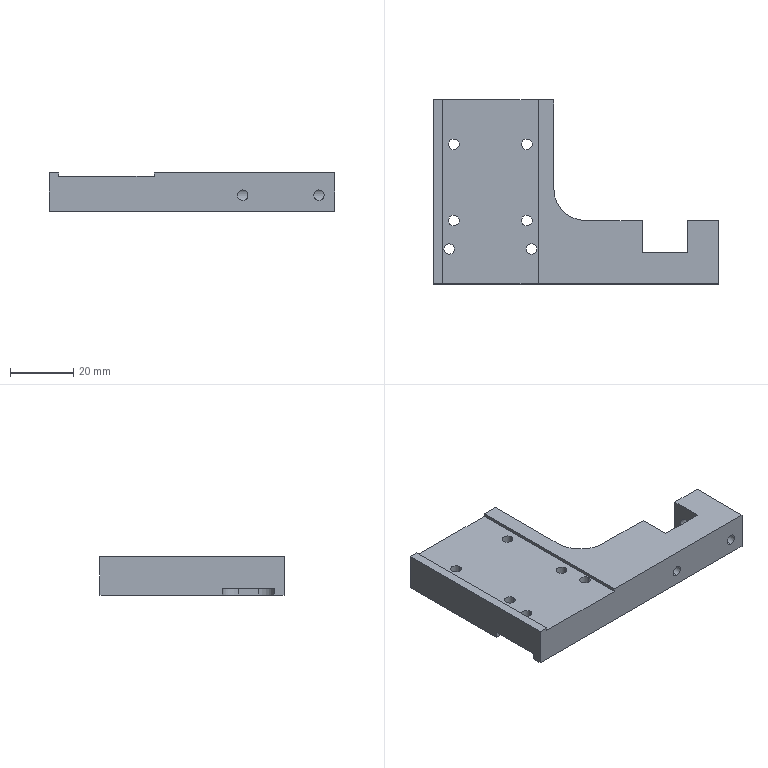Part | STEP file | PN_0010 Mount electronic clip quantitative slide block | 1 solid | 58 faces | box 90 x 58 x 12 mm | volume 32694 mm3 | cylinder 31 | plane 27 | commonest cylinder face diameters 3.3 x8 3.4 x8 6 x8 5 x4 10 x2 20 x1